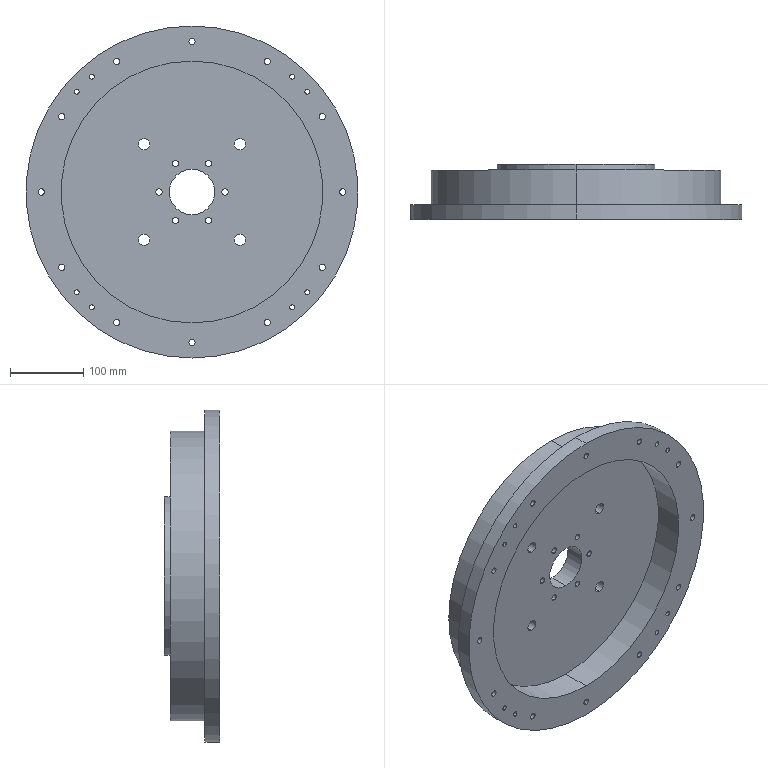Part | STEP file | 1 solid | 78 faces | box 452 x 75.25 x 452 mm | volume 5130306 mm3 | cylinder 72 | plane 6 | commonest cylinder face diameters 8.5 x36 6.5 x16 15.5 x8 62 x2 108 x2 215.9 x2